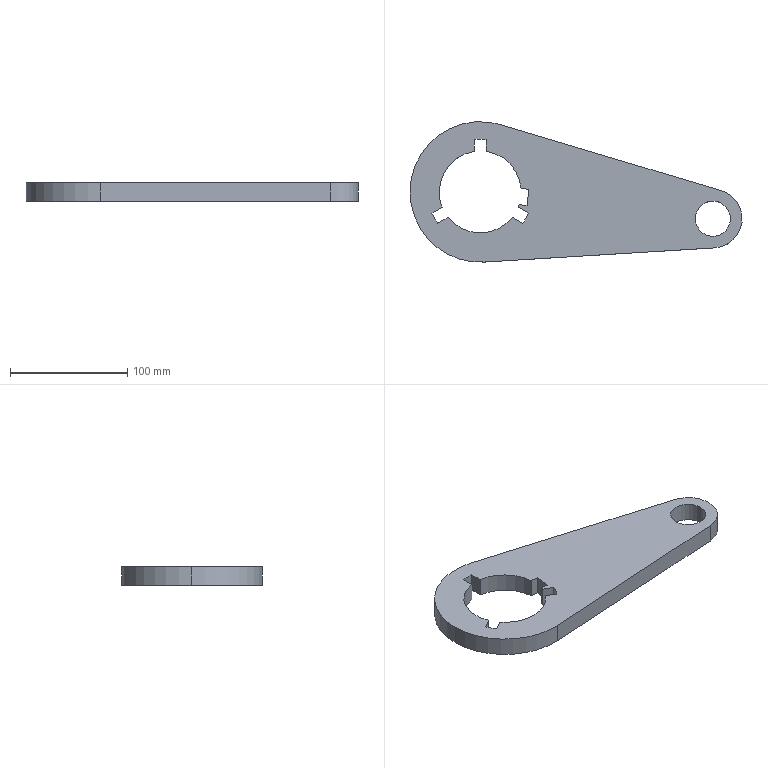Part | SolidWorks | features BaseBody 1 | 1 solid | 26 faces | box 283.692 x 120 x 16 mm | volume 303267 mm3 | cylinder 13 | plane 13 | commonest cylinder face diameters 70 x5 90 x3 30 x2 120 x2 50 x1
STEP:
#1=CARTESIAN_POINT('',(3286.241,1675.033,8.));
#2=VERTEX_POINT('',#1);
#3=CARTESIAN_POINT('',(3316.241,1675.033,8.));
#4=VERTEX_POINT('',#3);
#5=CARTESIAN_POINT('',(3301.241,1675.033,8.));
#6=DIRECTION('',(0.,0.,1.));
#7=DIRECTION('',(1.,0.,0.));
#8=AXIS2_PLACEMENT_3D('',#5,#6,#7);
#9=CIRCLE('',#8,15.);
#10=EDGE_CURVE('',#2,#4,#9,.T.);
#11=ORIENTED_EDGE('',*,*,#10,.T.);
#12=CARTESIAN_POINT('',(3316.241,1675.033,-8.));
#13=VERTEX_POINT('',#12);
#14=CARTESIAN_POINT('',(3316.241,1675.033,8.));
#15=DIRECTION('',(0.,0.,-1.));
#16=VECTOR('',#15,1000.);
#17=LINE('',#14,#16);
#18=EDGE_CURVE('',#4,#13,#17,.T.);
#19=ORIENTED_EDGE('',*,*,#18,.T.);
#20=CARTESIAN_POINT('',(3286.241,1675.033,-8.));
#21=VERTEX_POINT('',#20);
#22=CARTESIAN_POINT('',(3301.241,1675.033,-8.));
#23=DIRECTION('',(0.,0.,1.));
#24=DIRECTION('',(1.,0.,0.));
#25=AXIS2_PLACEMENT_3D('',#22,#23,#24);
#26=CIRCLE('',#25,15.);
#27=EDGE_CURVE('',#21,#13,#26,.T.);
#28=ORIENTED_EDGE('',*,*,#27,.F.);
#29=CARTESIAN_POINT('',(3286.241,1675.033,8.));
#30=DIRECTION('',(0.,0.,-1.));
#31=VECTOR('',#30,1000.);
#32=LINE('',#29,#31);
#33=EDGE_CURVE('',#2,#21,#32,.T.);
#34=ORIENTED_EDGE('',*,*,#33,.F.);
#35=EDGE_LOOP('',(#11,#19,#28,#34));
#36=FACE_OUTER_BOUND('',#35,.T.);
#37=CARTESIAN_POINT('',(3301.241,1675.033,8.));
#38=DIRECTION('',(0.,0.,-1.));
#39=DIRECTION('',(-1.,0.,0.));
#40=AXIS2_PLACEMENT_3D('',#37,#38,#39);
#41=CYLINDRICAL_SURFACE('',#40,15.);
#42=ADVANCED_FACE('',(#36),#41,.F.);
#43=CARTESIAN_POINT('',(3097.549,1732.51,8.));
#44=VERTEX_POINT('',#43);
#45=CARTESIAN_POINT('',(3067.549,1697.869,8.));
#46=VERTEX_POINT('',#45);
#47=CARTESIAN_POINT('',(3102.549,1697.869,8.));
#48=DIRECTION('',(0.,0.,1.));
#49=DIRECTION('',(1.,0.,0.));
#50=AXIS2_PLACEMENT_3D('',#47,#48,#49);
#51=CIRCLE('',#50,35.);
#52=EDGE_CURVE('',#44,#46,#51,.T.);
#53=ORIENTED_EDGE('',*,*,#52,.T.);
#54=CARTESIAN_POINT('',(3067.549,1697.869,-8.));
#55=VERTEX_POINT('',#54);
#56=CARTESIAN_POINT('',(3067.549,1697.869,8.));
#57=DIRECTION('',(0.,0.,-1.));
#58=VECTOR('',#57,1000.);
#59=LINE('',#56,#58);
#60=EDGE_CURVE('',#46,#55,#59,.T.);
#61=ORIENTED_EDGE('',*,*,#60,.T.);
#62=CARTESIAN_POINT('',(3097.549,1732.51,-8.));
#63=VERTEX_POINT('',#62);
#64=CARTESIAN_POINT('',(3102.549,1697.869,-8.));
#65=DIRECTION('',(0.,0.,1.));
#66=DIRECTION('',(1.,0.,0.));
#67=AXIS2_PLACEMENT_3D('',#64,#65,#66);
#68=CIRCLE('',#67,35.);
#69=EDGE_CURVE('',#63,#55,#68,.T.);
#70=ORIENTED_EDGE('',*,*,#69,.F.);
#71=CARTESIAN_POINT('',(3097.549,1732.51,8.));
#72=DIRECTION('',(0.,0.,-1.));
#73=VECTOR('',#72,1000.);
#74=LINE('',#71,#73);
#75=EDGE_CURVE('',#44,#63,#74,.T.);
#76=ORIENTED_EDGE('',*,*,#75,.F.);
#77=EDGE_LOOP('',(#53,#61,#70,#76));
#78=FACE_OUTER_BOUND('',#77,.T.);
#79=CARTESIAN_POINT('',(3102.549,1697.869,8.));
#80=DIRECTION('',(0.,0.,-1.));
#81=DIRECTION('',(-1.,0.,0.));
#82=AXIS2_PLACEMENT_3D('',#79,#80,#81);
#83=CYLINDRICAL_SURFACE('',#82,35.);
#84=ADVANCED_FACE('',(#78),#83,.F.);
#85=CARTESIAN_POINT('',(3042.549,1697.869,8.));
#86=VERTEX_POINT('',#85);
#87=CARTESIAN_POINT('',(3106.236,1637.983,8.));
#88=VERTEX_POINT('',#87);
#89=CARTESIAN_POINT('',(3102.549,1697.869,8.));
#90=DIRECTION('',(0.,0.,1.));
#91=DIRECTION('',(1.,0.,0.));
#92=AXIS2_PLACEMENT_3D('',#89,#90,#91);
#93=CIRCLE('',#92,60.);
#94=EDGE_CURVE('',#86,#88,#93,.T.);
#95=ORIENTED_EDGE('',*,*,#94,.F.);
#96=CARTESIAN_POINT('',(3042.549,1697.869,-8.));
#97=VERTEX_POINT('',#96);
#98=CARTESIAN_POINT('',(3042.549,1697.869,8.));
#99=DIRECTION('',(0.,0.,-1.));
#100=VECTOR('',#99,1000.);
#101=LINE('',#98,#100);
#102=EDGE_CURVE('',#86,#97,#101,.T.);
#103=ORIENTED_EDGE('',*,*,#102,.T.);
#104=CARTESIAN_POINT('',(3106.236,1637.983,-8.));
#105=VERTEX_POINT('',#104);
#106=CARTESIAN_POINT('',(3102.549,1697.869,-8.));
#107=DIRECTION('',(0.,0.,1.));
#108=DIRECTION('',(1.,0.,0.));
#109=AXIS2_PLACEMENT_3D('',#106,#107,#108);
#110=CIRCLE('',#109,60.);
#111=EDGE_CURVE('',#97,#105,#110,.T.);
#112=ORIENTED_EDGE('',*,*,#111,.T.);
#113=CARTESIAN_POINT('',(3106.236,1637.983,8.));
#114=DIRECTION('',(0.,0.,-1.));
#115=VECTOR('',#114,1000.);
#116=LINE('',#113,#115);
#117=EDGE_CURVE('',#88,#105,#116,.T.);
#118=ORIENTED_EDGE('',*,*,#117,.F.);
#119=EDGE_LOOP('',(#95,#103,#112,#118));
#120=FACE_OUTER_BOUND('',#119,.T.);
#121=CARTESIAN_POINT('',(3102.549,1697.869,8.));
#122=DIRECTION('',(0.,0.,-1.));
#123=DIRECTION('',(-1.,0.,0.));
#124=AXIS2_PLACEMENT_3D('',#121,#122,#123);
#125=CYLINDRICAL_SURFACE('',#124,60.);
#126=ADVANCED_FACE('',(#120),#125,.T.);
#127=CARTESIAN_POINT('',(3308.398,1698.987,-8.));
#128=VERTEX_POINT('',#127);
#129=CARTESIAN_POINT('',(3119.726,1755.358,-8.));
#130=VERTEX_POINT('',#129);
#131=CARTESIAN_POINT('',(737.152,2467.22,-8.));
#132=DIRECTION('',(-0.9581,0.2863,0.));
#133=VECTOR('',#132,1000.);
#134=LINE('',#131,#133);
#135=EDGE_CURVE('',#128,#130,#134,.T.);
#136=ORIENTED_EDGE('',*,*,#135,.T.);
#137=CARTESIAN_POINT('',(3119.726,1755.358,8.));
#138=VERTEX_POINT('',#137);
#139=CARTESIAN_POINT('',(3119.726,1755.358,8.));
#140=DIRECTION('',(0.,0.,-1.));
#141=VECTOR('',#140,1000.);
#142=LINE('',#139,#141);
#143=EDGE_CURVE('',#138,#130,#142,.T.);
#144=ORIENTED_EDGE('',*,*,#143,.F.);
#145=CARTESIAN_POINT('',(3308.398,1698.987,8.));
#146=VERTEX_POINT('',#145);
#147=CARTESIAN_POINT('',(737.152,2467.22,8.));
#148=DIRECTION('',(-0.9581,0.2863,0.));
#149=VECTOR('',#148,1000.);
#150=LINE('',#147,#149);
#151=EDGE_CURVE('',#146,#138,#150,.T.);
#152=ORIENTED_EDGE('',*,*,#151,.F.);
#153=CARTESIAN_POINT('',(3308.398,1698.987,8.));
#154=DIRECTION('',(0.,0.,-1.));
#155=VECTOR('',#154,1000.);
#156=LINE('',#153,#155);
#157=EDGE_CURVE('',#146,#128,#156,.T.);
#158=ORIENTED_EDGE('',*,*,#157,.T.);
#159=EDGE_LOOP('',(#136,#144,#152,#158));
#160=FACE_OUTER_BOUND('',#159,.T.);
#161=CARTESIAN_POINT('',(737.152,2467.22,8.));
#162=DIRECTION('',(-0.2863,-0.9581,0.));
#163=DIRECTION('',(0.9581,-0.2863,0.));
#164=AXIS2_PLACEMENT_3D('',#161,#162,#163);
#165=PLANE('',#164);
#166=ADVANCED_FACE('',(#160),#165,.F.);
#167=ORIENTED_EDGE('',*,*,#102,.F.);
#168=CARTESIAN_POINT('',(3102.549,1697.869,8.));
#169=DIRECTION('',(0.,0.,1.));
#170=DIRECTION('',(1.,0.,0.));
#171=AXIS2_PLACEMENT_3D('',#168,#169,#170);
#172=CIRCLE('',#171,60.);
#173=EDGE_CURVE('',#138,#86,#172,.T.);
#174=ORIENTED_EDGE('',*,*,#173,.F.);
#175=ORIENTED_EDGE('',*,*,#143,.T.);
#176=CARTESIAN_POINT('',(3102.549,1697.869,-8.));
#177=DIRECTION('',(0.,0.,1.));
#178=DIRECTION('',(1.,0.,0.));
#179=AXIS2_PLACEMENT_3D('',#176,#177,#178);
#180=CIRCLE('',#179,60.);
#181=EDGE_CURVE('',#130,#97,#180,.T.);
#182=ORIENTED_EDGE('',*,*,#181,.T.);
#183=EDGE_LOOP('',(#167,#174,#175,#182));
#184=FACE_OUTER_BOUND('',#183,.T.);
#185=CARTESIAN_POINT('',(3102.549,1697.869,8.));
#186=DIRECTION('',(0.,0.,-1.));
#187=DIRECTION('',(-1.,0.,0.));
#188=AXIS2_PLACEMENT_3D('',#185,#186,#187);
#189=CYLINDRICAL_SURFACE('',#188,60.);
#190=ADVANCED_FACE('',(#184),#189,.T.);
#191=CARTESIAN_POINT('',(3302.777,1650.081,-8.));
#192=VERTEX_POINT('',#191);
#193=CARTESIAN_POINT('',(-88.718,1441.323,-8.));
#194=DIRECTION('',(0.9981,0.06144,0.));
#195=VECTOR('',#194,1000.);
#196=LINE('',#193,#195);
#197=EDGE_CURVE('',#105,#192,#196,.T.);
#198=ORIENTED_EDGE('',*,*,#197,.T.);
#199=CARTESIAN_POINT('',(3302.777,1650.081,8.));
#200=VERTEX_POINT('',#199);
#201=CARTESIAN_POINT('',(3302.777,1650.081,8.));
#202=DIRECTION('',(0.,0.,-1.));
#203=VECTOR('',#202,1000.);
#204=LINE('',#201,#203);
#205=EDGE_CURVE('',#200,#192,#204,.T.);
#206=ORIENTED_EDGE('',*,*,#205,.F.);
#207=CARTESIAN_POINT('',(-88.718,1441.323,8.));
#208=DIRECTION('',(0.9981,0.06144,0.));
#209=VECTOR('',#208,1000.);
#210=LINE('',#207,#209);
#211=EDGE_CURVE('',#88,#200,#210,.T.);
#212=ORIENTED_EDGE('',*,*,#211,.F.);
#213=ORIENTED_EDGE('',*,*,#117,.T.);
#214=EDGE_LOOP('',(#198,#206,#212,#213));
#215=FACE_OUTER_BOUND('',#214,.T.);
#216=CARTESIAN_POINT('',(-88.718,1441.323,8.));
#217=DIRECTION('',(-0.06144,0.9981,0.));
#218=DIRECTION('',(-0.9981,-0.06144,0.));
#219=AXIS2_PLACEMENT_3D('',#216,#217,#218);
#220=PLANE('',#219);
#221=ADVANCED_FACE('',(#215),#220,.F.);
#222=CARTESIAN_POINT('',(3107.549,1742.591,-8.));
#223=VERTEX_POINT('',#222);
#224=CARTESIAN_POINT('',(3097.549,1742.591,-8.));
#225=VERTEX_POINT('',#224);
#226=CARTESIAN_POINT('',(3102.549,1697.869,-8.));
#227=DIRECTION('',(0.,0.,1.));
#228=DIRECTION('',(1.,0.,0.));
#229=AXIS2_PLACEMENT_3D('',#226,#227,#228);
#230=CIRCLE('',#229,45.);
#231=EDGE_CURVE('',#223,#225,#230,.T.);
#232=ORIENTED_EDGE('',*,*,#231,.F.);
#233=CARTESIAN_POINT('',(3107.549,1742.591,8.));
#234=VERTEX_POINT('',#233);
#235=CARTESIAN_POINT('',(3107.549,1742.591,8.));
#236=DIRECTION('',(0.,0.,-1.));
#237=VECTOR('',#236,1000.);
#238=LINE('',#235,#237);
#239=EDGE_CURVE('',#234,#223,#238,.T.);
#240=ORIENTED_EDGE('',*,*,#239,.F.);
#241=CARTESIAN_POINT('',(3097.549,1742.591,8.));
#242=VERTEX_POINT('',#241);
#243=CARTESIAN_POINT('',(3102.549,1697.869,8.));
#244=DIRECTION('',(0.,0.,1.));
#245=DIRECTION('',(1.,0.,0.));
#246=AXIS2_PLACEMENT_3D('',#243,#244,#245);
#247=CIRCLE('',#246,45.);
#248=EDGE_CURVE('',#234,#242,#247,.T.);
#249=ORIENTED_EDGE('',*,*,#248,.T.);
#250=CARTESIAN_POINT('',(3097.549,1742.591,8.));
#251=DIRECTION('',(0.,0.,-1.));
#252=VECTOR('',#251,1000.);
#253=LINE('',#250,#252);
#254=EDGE_CURVE('',#242,#225,#253,.T.);
#255=ORIENTED_EDGE('',*,*,#254,.T.);
#256=EDGE_LOOP('',(#232,#240,#249,#255));
#257=FACE_OUTER_BOUND('',#256,.T.);
#258=CARTESIAN_POINT('',(3102.549,1697.869,8.));
#259=DIRECTION('',(0.,0.,-1.));
#260=DIRECTION('',(-1.,0.,0.));
#261=AXIS2_PLACEMENT_3D('',#258,#259,#260);
#262=CYLINDRICAL_SURFACE('',#261,45.);
#263=ADVANCED_FACE('',(#257),#262,.F.);
#264=CARTESIAN_POINT('',(3107.549,1732.51,-8.));
#265=VERTEX_POINT('',#264);
#266=CARTESIAN_POINT('',(3107.549,0.,-8.));
#267=DIRECTION('',(0.,-1.,0.));
#268=VECTOR('',#267,1000.);
#269=LINE('',#266,#268);
#270=EDGE_CURVE('',#223,#265,#269,.T.);
#271=ORIENTED_EDGE('',*,*,#270,.T.);
#272=CARTESIAN_POINT('',(3107.549,1732.51,8.));
#273=VERTEX_POINT('',#272);
#274=CARTESIAN_POINT('',(3107.549,1732.51,8.));
#275=DIRECTION('',(0.,0.,-1.));
#276=VECTOR('',#275,1000.);
#277=LINE('',#274,#276);
#278=EDGE_CURVE('',#273,#265,#277,.T.);
#279=ORIENTED_EDGE('',*,*,#278,.F.);
#280=CARTESIAN_POINT('',(3107.549,0.,8.));
#281=DIRECTION('',(0.,-1.,0.));
#282=VECTOR('',#281,1000.);
#283=LINE('',#280,#282);
#284=EDGE_CURVE('',#234,#273,#283,.T.);
#285=ORIENTED_EDGE('',*,*,#284,.F.);
#286=ORIENTED_EDGE('',*,*,#239,.T.);
#287=EDGE_LOOP('',(#271,#279,#285,#286));
#288=FACE_OUTER_BOUND('',#287,.T.);
#289=CARTESIAN_POINT('',(3107.549,0.,8.));
#290=DIRECTION('',(1.,0.,0.));
#291=DIRECTION('',(0.,0.,-1.));
#292=AXIS2_PLACEMENT_3D('',#289,#290,#291);
#293=PLANE('',#292);
#294=ADVANCED_FACE('',(#288),#293,.F.);
#295=CARTESIAN_POINT('',(3137.417,1700.908,-8.));
#296=VERTEX_POINT('',#295);
#297=CARTESIAN_POINT('',(3102.549,1697.869,-8.));
#298=DIRECTION('',(0.,0.,1.));
#299=DIRECTION('',(1.,0.,0.));
#300=AXIS2_PLACEMENT_3D('',#297,#298,#299);
#301=CIRCLE('',#300,35.);
#302=EDGE_CURVE('',#296,#265,#301,.T.);
#303=ORIENTED_EDGE('',*,*,#302,.F.);
#304=CARTESIAN_POINT('',(3137.417,1700.908,8.));
#305=VERTEX_POINT('',#304);
#306=CARTESIAN_POINT('',(3137.417,1700.908,8.));
#307=DIRECTION('',(0.,0.,-1.));
#308=VECTOR('',#307,1000.);
#309=LINE('',#306,#308);
#310=EDGE_CURVE('',#305,#296,#309,.T.);
#311=ORIENTED_EDGE('',*,*,#310,.F.);
#312=CARTESIAN_POINT('',(3102.549,1697.869,8.));
#313=DIRECTION('',(0.,0.,1.));
#314=DIRECTION('',(1.,0.,0.));
#315=AXIS2_PLACEMENT_3D('',#312,#313,#314);
#316=CIRCLE('',#315,35.);
#317=EDGE_CURVE('',#305,#273,#316,.T.);
#318=ORIENTED_EDGE('',*,*,#317,.T.);
#319=ORIENTED_EDGE('',*,*,#278,.T.);
#320=EDGE_LOOP('',(#303,#311,#318,#319));
#321=FACE_OUTER_BOUND('',#320,.T.);
#322=CARTESIAN_POINT('',(3102.549,1697.869,8.));
#323=DIRECTION('',(0.,0.,-1.));
#324=DIRECTION('',(-1.,0.,0.));
#325=AXIS2_PLACEMENT_3D('',#322,#323,#324);
#326=CYLINDRICAL_SURFACE('',#325,35.);
#327=ADVANCED_FACE('',(#321),#326,.F.);
#328=CARTESIAN_POINT('',(3144.081,1700.142,-8.));
#329=VERTEX_POINT('',#328);
#330=CARTESIAN_POINT('',(233.843,2034.622,-8.));
#331=DIRECTION('',(0.9935,-0.1142,0.));
#332=VECTOR('',#331,1000.);
#333=LINE('',#330,#332);
#334=EDGE_CURVE('',#296,#329,#333,.T.);
#335=ORIENTED_EDGE('',*,*,#334,.T.);
#336=CARTESIAN_POINT('',(3144.081,1700.142,8.));
#337=VERTEX_POINT('',#336);
#338=CARTESIAN_POINT('',(3144.081,1700.142,8.));
#339=DIRECTION('',(0.,0.,-1.));
#340=VECTOR('',#339,1000.);
#341=LINE('',#338,#340);
#342=EDGE_CURVE('',#337,#329,#341,.T.);
#343=ORIENTED_EDGE('',*,*,#342,.F.);
#344=CARTESIAN_POINT('',(233.843,2034.622,8.));
#345=DIRECTION('',(0.9935,-0.1142,0.));
#346=VECTOR('',#345,1000.);
#347=LINE('',#344,#346);
#348=EDGE_CURVE('',#305,#337,#347,.T.);
#349=ORIENTED_EDGE('',*,*,#348,.F.);
#350=ORIENTED_EDGE('',*,*,#310,.T.);
#351=EDGE_LOOP('',(#335,#343,#349,#350));
#352=FACE_OUTER_BOUND('',#351,.T.);
#353=CARTESIAN_POINT('',(233.843,2034.622,8.));
#354=DIRECTION('',(0.1142,0.9935,0.));
#355=DIRECTION('',(-0.9935,0.1142,0.));
#356=AXIS2_PLACEMENT_3D('',#353,#354,#355);
#357=PLANE('',#356);
#358=ADVANCED_FACE('',(#352),#357,.F.);
#359=CARTESIAN_POINT('',(3142.482,1686.234,-8.));
#360=VERTEX_POINT('',#359);
#361=CARTESIAN_POINT('',(2910.237,-334.48,-8.));
#362=DIRECTION('',(0.1142,0.9935,0.));
#363=VECTOR('',#362,1000.);
#364=LINE('',#361,#363);
#365=EDGE_CURVE('',#360,#329,#364,.T.);
#366=ORIENTED_EDGE('',*,*,#365,.F.);
#367=CARTESIAN_POINT('',(3142.482,1686.234,8.));
#368=VERTEX_POINT('',#367);
#369=CARTESIAN_POINT('',(3142.482,1686.234,8.));
#370=DIRECTION('',(0.,0.,-1.));
#371=VECTOR('',#370,1000.);
#372=LINE('',#369,#371);
#373=EDGE_CURVE('',#368,#360,#372,.T.);
#374=ORIENTED_EDGE('',*,*,#373,.F.);
#375=CARTESIAN_POINT('',(2910.237,-334.48,8.));
#376=DIRECTION('',(0.1142,0.9935,0.));
#377=VECTOR('',#376,1000.);
#378=LINE('',#375,#377);
#379=EDGE_CURVE('',#368,#337,#378,.T.);
#380=ORIENTED_EDGE('',*,*,#379,.T.);
#381=ORIENTED_EDGE('',*,*,#342,.T.);
#382=EDGE_LOOP('',(#366,#374,#380,#381));
#383=FACE_OUTER_BOUND('',#382,.T.);
#384=CARTESIAN_POINT('',(2910.237,-334.48,8.));
#385=DIRECTION('',(-0.9935,0.1142,0.));
#386=DIRECTION('',(-0.1142,-0.9935,0.));
#387=AXIS2_PLACEMENT_3D('',#384,#385,#386);
#388=PLANE('',#387);
#389=ADVANCED_FACE('',(#383),#388,.T.);
#390=CARTESIAN_POINT('',(3135.819,1687.,-8.));
#391=VERTEX_POINT('',#390);
#392=CARTESIAN_POINT('',(232.245,2020.713,-8.));
#393=DIRECTION('',(0.9935,-0.1142,0.));
#394=VECTOR('',#393,1000.);
#395=LINE('',#392,#394);
#396=EDGE_CURVE('',#391,#360,#395,.T.);
#397=ORIENTED_EDGE('',*,*,#396,.F.);
#398=CARTESIAN_POINT('',(3135.819,1687.,8.));
#399=VERTEX_POINT('',#398);
#400=CARTESIAN_POINT('',(3135.819,1687.,8.));
#401=DIRECTION('',(0.,0.,-1.));
#402=VECTOR('',#401,1000.);
#403=LINE('',#400,#402);
#404=EDGE_CURVE('',#399,#391,#403,.T.);
#405=ORIENTED_EDGE('',*,*,#404,.F.);
#406=CARTESIAN_POINT('',(232.245,2020.713,8.));
#407=DIRECTION('',(0.9935,-0.1142,0.));
#408=VECTOR('',#407,1000.);
#409=LINE('',#406,#408);
#410=EDGE_CURVE('',#399,#368,#409,.T.);
#411=ORIENTED_EDGE('',*,*,#410,.T.);
#412=ORIENTED_EDGE('',*,*,#373,.T.);
#413=EDGE_LOOP('',(#397,#405,#411,#412));
#414=FACE_OUTER_BOUND('',#413,.T.);
#415=CARTESIAN_POINT('',(232.245,2020.713,8.));
#416=DIRECTION('',(0.1142,0.9935,0.));
#417=DIRECTION('',(-0.9935,0.1142,0.));
#418=AXIS2_PLACEMENT_3D('',#415,#416,#417);
#419=PLANE('',#418);
#420=ADVANCED_FACE('',(#414),#419,.T.);
#421=CARTESIAN_POINT('',(3135.049,1684.879,-8.));
#422=VERTEX_POINT('',#421);
#423=CARTESIAN_POINT('',(3102.549,1697.869,-8.));
#424=DIRECTION('',(0.,0.,1.));
#425=DIRECTION('',(1.,0.,0.));
#426=AXIS2_PLACEMENT_3D('',#423,#424,#425);
#427=CIRCLE('',#426,35.);
#428=EDGE_CURVE('',#422,#391,#427,.T.);
#429=ORIENTED_EDGE('',*,*,#428,.F.);
#430=CARTESIAN_POINT('',(3135.049,1684.879,8.));
#431=VERTEX_POINT('',#430);
#432=CARTESIAN_POINT('',(3135.049,1684.879,8.));
#433=DIRECTION('',(0.,0.,-1.));
#434=VECTOR('',#433,1000.);
#435=LINE('',#432,#434);
#436=EDGE_CURVE('',#431,#422,#435,.T.);
#437=ORIENTED_EDGE('',*,*,#436,.F.);
#438=CARTESIAN_POINT('',(3102.549,1697.869,8.));
#439=DIRECTION('',(0.,0.,1.));
#440=DIRECTION('',(1.,0.,0.));
#441=AXIS2_PLACEMENT_3D('',#438,#439,#440);
#442=CIRCLE('',#441,35.);
#443=EDGE_CURVE('',#431,#399,#442,.T.);
#444=ORIENTED_EDGE('',*,*,#443,.T.);
#445=ORIENTED_EDGE('',*,*,#404,.T.);
#446=EDGE_LOOP('',(#429,#437,#444,#445));
#447=FACE_OUTER_BOUND('',#446,.T.);
#448=CARTESIAN_POINT('',(3102.549,1697.869,8.));
#449=DIRECTION('',(0.,0.,-1.));
#450=DIRECTION('',(-1.,0.,0.));
#451=AXIS2_PLACEMENT_3D('',#448,#449,#450);
#452=CYLINDRICAL_SURFACE('',#451,35.);
#453=ADVANCED_FACE('',(#447),#452,.F.);
#454=CARTESIAN_POINT('',(3143.779,1679.839,-8.));
#455=VERTEX_POINT('',#454);
#456=CARTESIAN_POINT('',(1513.336,2621.176,-8.));
#457=DIRECTION('',(-0.866,0.5,0.));
#458=VECTOR('',#457,1000.);
#459=LINE('',#456,#458);
#460=EDGE_CURVE('',#455,#422,#459,.T.);
#461=ORIENTED_EDGE('',*,*,#460,.F.);
#462=CARTESIAN_POINT('',(3143.779,1679.839,8.));
#463=VERTEX_POINT('',#462);
#464=CARTESIAN_POINT('',(3143.779,1679.839,8.));
#465=DIRECTION('',(0.,0.,-1.));
#466=VECTOR('',#465,1000.);
#467=LINE('',#464,#466);
#468=EDGE_CURVE('',#463,#455,#467,.T.);
#469=ORIENTED_EDGE('',*,*,#468,.F.);
#470=CARTESIAN_POINT('',(1513.336,2621.176,8.));
#471=DIRECTION('',(-0.866,0.5,0.));
#472=VECTOR('',#471,1000.);
#473=LINE('',#470,#472);
#474=EDGE_CURVE('',#463,#431,#473,.T.);
#475=ORIENTED_EDGE('',*,*,#474,.T.);
#476=ORIENTED_EDGE('',*,*,#436,.T.);
#477=EDGE_LOOP('',(#461,#469,#475,#476));
#478=FACE_OUTER_BOUND('',#477,.T.);
#479=CARTESIAN_POINT('',(1513.336,2621.176,8.));
#480=DIRECTION('',(-0.5,-0.866,0.));
#481=DIRECTION('',(0.866,-0.5,0.));
#482=AXIS2_PLACEMENT_3D('',#479,#480,#481);
#483=PLANE('',#482);
#484=ADVANCED_FACE('',(#478),#483,.T.);
#485=CARTESIAN_POINT('',(3138.779,1671.179,-8.));
#486=VERTEX_POINT('',#485);
#487=CARTESIAN_POINT('',(3102.549,1697.869,-8.));
#488=DIRECTION('',(0.,0.,1.));
#489=DIRECTION('',(1.,0.,0.));
#490=AXIS2_PLACEMENT_3D('',#487,#488,#489);
#491=CIRCLE('',#490,45.);
#492=EDGE_CURVE('',#486,#455,#491,.T.);
#493=ORIENTED_EDGE('',*,*,#492,.F.);
#494=CARTESIAN_POINT('',(3138.779,1671.179,8.));
#495=VERTEX_POINT('',#494);
#496=CARTESIAN_POINT('',(3138.779,1671.179,8.));
#497=DIRECTION('',(0.,0.,-1.));
#498=VECTOR('',#497,1000.);
#499=LINE('',#496,#498);
#500=EDGE_CURVE('',#495,#486,#499,.T.);
#501=ORIENTED_EDGE('',*,*,#500,.F.);
#502=CARTESIAN_POINT('',(3102.549,1697.869,8.));
#503=DIRECTION('',(0.,0.,1.));
#504=DIRECTION('',(1.,0.,0.));
#505=AXIS2_PLACEMENT_3D('',#502,#503,#504);
#506=CIRCLE('',#505,45.);
#507=EDGE_CURVE('',#495,#463,#506,.T.);
#508=ORIENTED_EDGE('',*,*,#507,.T.);
#509=ORIENTED_EDGE('',*,*,#468,.T.);
#510=EDGE_LOOP('',(#493,#501,#508,#509));
#511=FACE_OUTER_BOUND('',#510,.T.);
#512=CARTESIAN_POINT('',(3102.549,1697.869,8.));
#513=DIRECTION('',(0.,0.,-1.));
#514=DIRECTION('',(-1.,0.,0.));
#515=AXIS2_PLACEMENT_3D('',#512,#513,#514);
#516=CYLINDRICAL_SURFACE('',#515,45.);
#517=ADVANCED_FACE('',(#511),#516,.F.);
#518=CARTESIAN_POINT('',(3130.049,1676.219,-8.));
#519=VERTEX_POINT('',#518);
#520=CARTESIAN_POINT('',(1508.336,2612.515,-8.));
#521=DIRECTION('',(-0.866,0.5,0.));
#522=VECTOR('',#521,1000.);
#523=LINE('',#520,#522);
#524=EDGE_CURVE('',#486,#519,#523,.T.);
#525=ORIENTED_EDGE('',*,*,#524,.T.);
#526=CARTESIAN_POINT('',(3130.049,1676.219,8.));
#527=VERTEX_POINT('',#526);
#528=CARTESIAN_POINT('',(3130.049,1676.219,8.));
#529=DIRECTION('',(0.,0.,-1.));
#530=VECTOR('',#529,1000.);
#531=LINE('',#528,#530);
#532=EDGE_CURVE('',#527,#519,#531,.T.);
#533=ORIENTED_EDGE('',*,*,#532,.F.);
#534=CARTESIAN_POINT('',(1508.336,2612.515,8.));
#535=DIRECTION('',(-0.866,0.5,0.));
#536=VECTOR('',#535,1000.);
#537=LINE('',#534,#536);
#538=EDGE_CURVE('',#495,#527,#537,.T.);
#539=ORIENTED_EDGE('',*,*,#538,.F.);
#540=ORIENTED_EDGE('',*,*,#500,.T.);
#541=EDGE_LOOP('',(#525,#533,#539,#540));
#542=FACE_OUTER_BOUND('',#541,.T.);
#543=CARTESIAN_POINT('',(1508.336,2612.515,8.));
#544=DIRECTION('',(-0.5,-0.866,0.));
#545=DIRECTION('',(0.866,-0.5,0.));
#546=AXIS2_PLACEMENT_3D('',#543,#544,#545);
#547=PLANE('',#546);
#548=ADVANCED_FACE('',(#542),#547,.F.);
#549=CARTESIAN_POINT('',(3075.049,1676.219,-8.));
#550=VERTEX_POINT('',#549);
#551=CARTESIAN_POINT('',(3102.549,1697.869,-8.));
#552=DIRECTION('',(0.,0.,1.));
#553=DIRECTION('',(1.,0.,0.));
#554=AXIS2_PLACEMENT_3D('',#551,#552,#553);
#555=CIRCLE('',#554,35.);
#556=EDGE_CURVE('',#550,#519,#555,.T.);
#557=ORIENTED_EDGE('',*,*,#556,.F.);
#558=CARTESIAN_POINT('',(3075.049,1676.219,8.));
#559=VERTEX_POINT('',#558);
#560=CARTESIAN_POINT('',(3075.049,1676.219,8.));
#561=DIRECTION('',(0.,0.,-1.));
#562=VECTOR('',#561,1000.);
#563=LINE('',#560,#562);
#564=EDGE_CURVE('',#559,#550,#563,.T.);
#565=ORIENTED_EDGE('',*,*,#564,.F.);
#566=CARTESIAN_POINT('',(3102.549,1697.869,8.));
#567=DIRECTION('',(0.,0.,1.));
#568=DIRECTION('',(1.,0.,0.));
#569=AXIS2_PLACEMENT_3D('',#566,#567,#568);
#570=CIRCLE('',#569,35.);
#571=EDGE_CURVE('',#559,#527,#570,.T.);
#572=ORIENTED_EDGE('',*,*,#571,.T.);
#573=ORIENTED_EDGE('',*,*,#532,.T.);
#574=EDGE_LOOP('',(#557,#565,#572,#573));
#575=FACE_OUTER_BOUND('',#574,.T.);
#576=CARTESIAN_POINT('',(3102.549,1697.869,8.));
#577=DIRECTION('',(0.,0.,-1.));
#578=DIRECTION('',(-1.,0.,0.));
#579=AXIS2_PLACEMENT_3D('',#576,#577,#578);
#580=CYLINDRICAL_SURFACE('',#579,35.);
#581=ADVANCED_FACE('',(#575),#580,.F.);
#582=CARTESIAN_POINT('',(3066.32,1671.179,-8.));
#583=VERTEX_POINT('',#582);
#584=CARTESIAN_POINT('',(42.938,-74.371,-8.));
#585=DIRECTION('',(0.866,0.5,0.));
#586=VECTOR('',#585,1000.);
#587=LINE('',#584,#586);
#588=EDGE_CURVE('',#583,#550,#587,.T.);
#589=ORIENTED_EDGE('',*,*,#588,.F.);
#590=CARTESIAN_POINT('',(3066.32,1671.179,8.));
#591=VERTEX_POINT('',#590);
#592=CARTESIAN_POINT('',(3066.32,1671.179,8.));
#593=DIRECTION('',(0.,0.,-1.));
#594=VECTOR('',#593,1000.);
#595=LINE('',#592,#594);
#596=EDGE_CURVE('',#591,#583,#595,.T.);
#597=ORIENTED_EDGE('',*,*,#596,.F.);
#598=CARTESIAN_POINT('',(42.938,-74.371,8.));
#599=DIRECTION('',(0.866,0.5,0.));
#600=VECTOR('',#599,1000.);
#601=LINE('',#598,#600);
#602=EDGE_CURVE('',#591,#559,#601,.T.);
#603=ORIENTED_EDGE('',*,*,#602,.T.);
#604=ORIENTED_EDGE('',*,*,#564,.T.);
#605=EDGE_LOOP('',(#589,#597,#603,#604));
#606=FACE_OUTER_BOUND('',#605,.T.);
#607=CARTESIAN_POINT('',(42.938,-74.371,8.));
#608=DIRECTION('',(-0.5,0.866,0.));
#609=DIRECTION('',(-0.866,-0.5,0.));
#610=AXIS2_PLACEMENT_3D('',#607,#608,#609);
#611=PLANE('',#610);
#612=ADVANCED_FACE('',(#606),#611,.T.);
#613=CARTESIAN_POINT('',(3061.32,1679.839,-8.));
#614=VERTEX_POINT('',#613);
#615=CARTESIAN_POINT('',(3102.549,1697.869,-8.));
#616=DIRECTION('',(0.,0.,1.));
#617=DIRECTION('',(1.,0.,0.));
#618=AXIS2_PLACEMENT_3D('',#615,#616,#617);
#619=CIRCLE('',#618,45.);
#620=EDGE_CURVE('',#614,#583,#619,.T.);
#621=ORIENTED_EDGE('',*,*,#620,.F.);
#622=CARTESIAN_POINT('',(3061.32,1679.839,8.));
#623=VERTEX_POINT('',#622);
#624=CARTESIAN_POINT('',(3061.32,1679.839,8.));
#625=DIRECTION('',(0.,0.,-1.));
#626=VECTOR('',#625,1000.);
#627=LINE('',#624,#626);
#628=EDGE_CURVE('',#623,#614,#627,.T.);
#629=ORIENTED_EDGE('',*,*,#628,.F.);
#630=CARTESIAN_POINT('',(3102.549,1697.869,8.));
#631=DIRECTION('',(0.,0.,1.));
#632=DIRECTION('',(1.,0.,0.));
#633=AXIS2_PLACEMENT_3D('',#630,#631,#632);
#634=CIRCLE('',#633,45.);
#635=EDGE_CURVE('',#623,#591,#634,.T.);
#636=ORIENTED_EDGE('',*,*,#635,.T.);
#637=ORIENTED_EDGE('',*,*,#596,.T.);
#638=EDGE_LOOP('',(#621,#629,#636,#637));
#639=FACE_OUTER_BOUND('',#638,.T.);
#640=CARTESIAN_POINT('',(3102.549,1697.869,8.));
#641=DIRECTION('',(0.,0.,-1.));
#642=DIRECTION('',(-1.,0.,0.));
#643=AXIS2_PLACEMENT_3D('',#640,#641,#642);
#644=CYLINDRICAL_SURFACE('',#643,45.);
#645=ADVANCED_FACE('',(#639),#644,.F.);
#646=CARTESIAN_POINT('',(3070.049,1684.879,-8.));
#647=VERTEX_POINT('',#646);
#648=CARTESIAN_POINT('',(37.938,-65.711,-8.));
#649=DIRECTION('',(0.866,0.5,0.));
#650=VECTOR('',#649,1000.);
#651=LINE('',#648,#650);
#652=EDGE_CURVE('',#614,#647,#651,.T.);
#653=ORIENTED_EDGE('',*,*,#652,.T.);
#654=CARTESIAN_POINT('',(3070.049,1684.879,8.));
#655=VERTEX_POINT('',#654);
#656=CARTESIAN_POINT('',(3070.049,1684.879,8.));
#657=DIRECTION('',(0.,0.,-1.));
#658=VECTOR('',#657,1000.);
#659=LINE('',#656,#658);
#660=EDGE_CURVE('',#655,#647,#659,.T.);
#661=ORIENTED_EDGE('',*,*,#660,.F.);
#662=CARTESIAN_POINT('',(37.938,-65.711,8.));
#663=DIRECTION('',(0.866,0.5,0.));
#664=VECTOR('',#663,1000.);
#665=LINE('',#662,#664);
#666=EDGE_CURVE('',#623,#655,#665,.T.);
#667=ORIENTED_EDGE('',*,*,#666,.F.);
#668=ORIENTED_EDGE('',*,*,#628,.T.);
#669=EDGE_LOOP('',(#653,#661,#667,#668));
#670=FACE_OUTER_BOUND('',#669,.T.);
#671=CARTESIAN_POINT('',(37.938,-65.711,8.));
#672=DIRECTION('',(-0.5,0.866,0.));
#673=DIRECTION('',(-0.866,-0.5,0.));
#674=AXIS2_PLACEMENT_3D('',#671,#672,#673);
#675=PLANE('',#674);
#676=ADVANCED_FACE('',(#670),#675,.F.);
#677=ORIENTED_EDGE('',*,*,#60,.F.);
#678=CARTESIAN_POINT('',(3102.549,1697.869,8.));
#679=DIRECTION('',(0.,0.,1.));
#680=DIRECTION('',(1.,0.,0.));
#681=AXIS2_PLACEMENT_3D('',#678,#679,#680);
#682=CIRCLE('',#681,35.);
#683=EDGE_CURVE('',#46,#655,#682,.T.);
#684=ORIENTED_EDGE('',*,*,#683,.T.);
#685=ORIENTED_EDGE('',*,*,#660,.T.);
#686=CARTESIAN_POINT('',(3102.549,1697.869,-8.));
#687=DIRECTION('',(0.,0.,1.));
#688=DIRECTION('',(1.,0.,0.));
#689=AXIS2_PLACEMENT_3D('',#686,#687,#688);
#690=CIRCLE('',#689,35.);
#691=EDGE_CURVE('',#55,#647,#690,.T.);
#692=ORIENTED_EDGE('',*,*,#691,.F.);
#693=EDGE_LOOP('',(#677,#684,#685,#692));
#694=FACE_OUTER_BOUND('',#693,.T.);
#695=CARTESIAN_POINT('',(3102.549,1697.869,8.));
#696=DIRECTION('',(0.,0.,-1.));
#697=DIRECTION('',(-1.,0.,0.));
#698=AXIS2_PLACEMENT_3D('',#695,#696,#697);
#699=CYLINDRICAL_SURFACE('',#698,35.);
#700=ADVANCED_FACE('',(#694),#699,.F.);
#701=ORIENTED_EDGE('',*,*,#18,.F.);
#702=CARTESIAN_POINT('',(3301.241,1675.033,8.));
#703=DIRECTION('',(0.,0.,1.));
#704=DIRECTION('',(1.,0.,0.));
#705=AXIS2_PLACEMENT_3D('',#702,#703,#704);
#706=CIRCLE('',#705,15.);
#707=EDGE_CURVE('',#4,#2,#706,.T.);
#708=ORIENTED_EDGE('',*,*,#707,.T.);
#709=ORIENTED_EDGE('',*,*,#33,.T.);
#710=CARTESIAN_POINT('',(3301.241,1675.033,-8.));
#711=DIRECTION('',(0.,0.,1.));
#712=DIRECTION('',(1.,0.,0.));
#713=AXIS2_PLACEMENT_3D('',#710,#711,#712);
#714=CIRCLE('',#713,15.);
#715=EDGE_CURVE('',#13,#21,#714,.T.);
#716=ORIENTED_EDGE('',*,*,#715,.F.);
#717=EDGE_LOOP('',(#701,#708,#709,#716));
#718=FACE_OUTER_BOUND('',#717,.T.);
#719=CARTESIAN_POINT('',(3301.241,1675.033,8.));
#720=DIRECTION('',(0.,0.,-1.));
#721=DIRECTION('',(-1.,0.,0.));
#722=AXIS2_PLACEMENT_3D('',#719,#720,#721);
#723=CYLINDRICAL_SURFACE('',#722,15.);
#724=ADVANCED_FACE('',(#718),#723,.F.);
#725=CARTESIAN_POINT('',(3097.549,0.,-8.));
#726=DIRECTION('',(0.,-1.,0.));
#727=VECTOR('',#726,1000.);
#728=LINE('',#725,#727);
#729=EDGE_CURVE('',#225,#63,#728,.T.);
#730=ORIENTED_EDGE('',*,*,#729,.F.);
#731=ORIENTED_EDGE('',*,*,#254,.F.);
#732=CARTESIAN_POINT('',(3097.549,0.,8.));
#733=DIRECTION('',(0.,-1.,0.));
#734=VECTOR('',#733,1000.);
#735=LINE('',#732,#734);
#736=EDGE_CURVE('',#242,#44,#735,.T.);
#737=ORIENTED_EDGE('',*,*,#736,.T.);
#738=ORIENTED_EDGE('',*,*,#75,.T.);
#739=EDGE_LOOP('',(#730,#731,#737,#738));
#740=FACE_OUTER_BOUND('',#739,.T.);
#741=CARTESIAN_POINT('',(3097.549,0.,8.));
#742=DIRECTION('',(1.,0.,0.));
#743=DIRECTION('',(0.,0.,-1.));
#744=AXIS2_PLACEMENT_3D('',#741,#742,#743);
#745=PLANE('',#744);
#746=ADVANCED_FACE('',(#740),#745,.T.);
#747=CARTESIAN_POINT('',(3301.241,1675.033,-8.));
#748=DIRECTION('',(0.,0.,1.));
#749=DIRECTION('',(1.,0.,0.));
#750=AXIS2_PLACEMENT_3D('',#747,#748,#749);
#751=CIRCLE('',#750,25.);
#752=EDGE_CURVE('',#192,#128,#751,.T.);
#753=ORIENTED_EDGE('',*,*,#752,.T.);
#754=ORIENTED_EDGE('',*,*,#157,.F.);
#755=CARTESIAN_POINT('',(3301.241,1675.033,8.));
#756=DIRECTION('',(0.,0.,1.));
#757=DIRECTION('',(1.,0.,0.));
#758=AXIS2_PLACEMENT_3D('',#755,#756,#757);
#759=CIRCLE('',#758,25.);
#760=EDGE_CURVE('',#200,#146,#759,.T.);
#761=ORIENTED_EDGE('',*,*,#760,.F.);
#762=ORIENTED_EDGE('',*,*,#205,.T.);
#763=EDGE_LOOP('',(#753,#754,#761,#762));
#764=FACE_OUTER_BOUND('',#763,.T.);
#765=CARTESIAN_POINT('',(3301.241,1675.033,8.));
#766=DIRECTION('',(0.,0.,-1.));
#767=DIRECTION('',(-1.,0.,0.));
#768=AXIS2_PLACEMENT_3D('',#765,#766,#767);
#769=CYLINDRICAL_SURFACE('',#768,25.);
#770=ADVANCED_FACE('',(#764),#769,.T.);
#771=ORIENTED_EDGE('',*,*,#248,.F.);
#772=ORIENTED_EDGE('',*,*,#284,.T.);
#773=ORIENTED_EDGE('',*,*,#317,.F.);
#774=ORIENTED_EDGE('',*,*,#348,.T.);
#775=ORIENTED_EDGE('',*,*,#379,.F.);
#776=ORIENTED_EDGE('',*,*,#410,.F.);
#777=ORIENTED_EDGE('',*,*,#443,.F.);
#778=ORIENTED_EDGE('',*,*,#474,.F.);
#779=ORIENTED_EDGE('',*,*,#507,.F.);
#780=ORIENTED_EDGE('',*,*,#538,.T.);
#781=ORIENTED_EDGE('',*,*,#571,.F.);
#782=ORIENTED_EDGE('',*,*,#602,.F.);
#783=ORIENTED_EDGE('',*,*,#635,.F.);
#784=ORIENTED_EDGE('',*,*,#666,.T.);
#785=ORIENTED_EDGE('',*,*,#683,.F.);
#786=ORIENTED_EDGE('',*,*,#52,.F.);
#787=ORIENTED_EDGE('',*,*,#736,.F.);
#788=EDGE_LOOP('',(#771,#772,#773,#774,#775,#776,#777,#778,#779,#780,#781,#782,#783,#784,#785,#786,#787));
#789=FACE_BOUND('',#788,.T.);
#790=ORIENTED_EDGE('',*,*,#10,.F.);
#791=ORIENTED_EDGE('',*,*,#707,.F.);
#792=EDGE_LOOP('',(#790,#791));
#793=FACE_BOUND('',#792,.T.);
#794=ORIENTED_EDGE('',*,*,#151,.T.);
#795=ORIENTED_EDGE('',*,*,#173,.T.);
#796=ORIENTED_EDGE('',*,*,#94,.T.);
#797=ORIENTED_EDGE('',*,*,#211,.T.);
#798=ORIENTED_EDGE('',*,*,#760,.T.);
#799=EDGE_LOOP('',(#794,#795,#796,#797,#798));
#800=FACE_OUTER_BOUND('',#799,.T.);
#801=CARTESIAN_POINT('',(0.,0.,8.));
#802=DIRECTION('',(0.,0.,1.));
#803=DIRECTION('',(1.,0.,0.));
#804=AXIS2_PLACEMENT_3D('',#801,#802,#803);
#805=PLANE('',#804);
#806=ADVANCED_FACE('',(#789,#793,#800),#805,.T.);
#807=ORIENTED_EDGE('',*,*,#231,.T.);
#808=ORIENTED_EDGE('',*,*,#729,.T.);
#809=ORIENTED_EDGE('',*,*,#69,.T.);
#810=ORIENTED_EDGE('',*,*,#691,.T.);
#811=ORIENTED_EDGE('',*,*,#652,.F.);
#812=ORIENTED_EDGE('',*,*,#620,.T.);
#813=ORIENTED_EDGE('',*,*,#588,.T.);
#814=ORIENTED_EDGE('',*,*,#556,.T.);
#815=ORIENTED_EDGE('',*,*,#524,.F.);
#816=ORIENTED_EDGE('',*,*,#492,.T.);
#817=ORIENTED_EDGE('',*,*,#460,.T.);
#818=ORIENTED_EDGE('',*,*,#428,.T.);
#819=ORIENTED_EDGE('',*,*,#396,.T.);
#820=ORIENTED_EDGE('',*,*,#365,.T.);
#821=ORIENTED_EDGE('',*,*,#334,.F.);
#822=ORIENTED_EDGE('',*,*,#302,.T.);
#823=ORIENTED_EDGE('',*,*,#270,.F.);
#824=EDGE_LOOP('',(#807,#808,#809,#810,#811,#812,#813,#814,#815,#816,#817,#818,#819,#820,#821,#822,#823));
#825=FACE_BOUND('',#824,.T.);
#826=ORIENTED_EDGE('',*,*,#27,.T.);
#827=ORIENTED_EDGE('',*,*,#715,.T.);
#828=EDGE_LOOP('',(#826,#827));
#829=FACE_BOUND('',#828,.T.);
#830=ORIENTED_EDGE('',*,*,#135,.F.);
#831=ORIENTED_EDGE('',*,*,#752,.F.);
#832=ORIENTED_EDGE('',*,*,#197,.F.);
#833=ORIENTED_EDGE('',*,*,#111,.F.);
#834=ORIENTED_EDGE('',*,*,#181,.F.);
#835=EDGE_LOOP('',(#830,#831,#832,#833,#834));
#836=FACE_OUTER_BOUND('',#835,.T.);
#837=CARTESIAN_POINT('',(0.,0.,-8.));
#838=DIRECTION('',(0.,0.,1.));
#839=DIRECTION('',(1.,0.,0.));
#840=AXIS2_PLACEMENT_3D('',#837,#838,#839);
#841=PLANE('',#840);
#842=ADVANCED_FACE('',(#825,#829,#836),#841,.F.);
#843=CLOSED_SHELL('',(#42,#84,#126,#166,#190,#221,#263,#294,#327,#358,#389,#420,#453,#484,#517,#548,#581,#612,#645,#676,#700,#724,#746,#770,#806,#842));
#844=MANIFOLD_SOLID_BREP('',#843);
#845=CARTESIAN_POINT('',(0.,0.,0.));
#846=DIRECTION('',(0.,0.,1.));
#847=DIRECTION('',(1.,0.,0.));
#848=AXIS2_PLACEMENT_3D('',#845,#846,#847);
#849=(LENGTH_UNIT()NAMED_UNIT(*)SI_UNIT(.MILLI.,.METRE.));
#850=UNCERTAINTY_MEASURE_WITH_UNIT(LENGTH_MEASURE(0.00001),#849,'','');
#851=(NAMED_UNIT(*)PLANE_ANGLE_UNIT()SI_UNIT($,.RADIAN.));
#852=(NAMED_UNIT(*)SI_UNIT($,.STERADIAN.)SOLID_ANGLE_UNIT());
#853=(GEOMETRIC_REPRESENTATION_CONTEXT(3)GLOBAL_UNCERTAINTY_ASSIGNED_CONTEXT((#850))GLOBAL_UNIT_ASSIGNED_CONTEXT((#849,#851,#852))REPRESENTATION_CONTEXT('',''));
#854=ADVANCED_BREP_SHAPE_REPRESENTATION('',(#844,#848),#853);